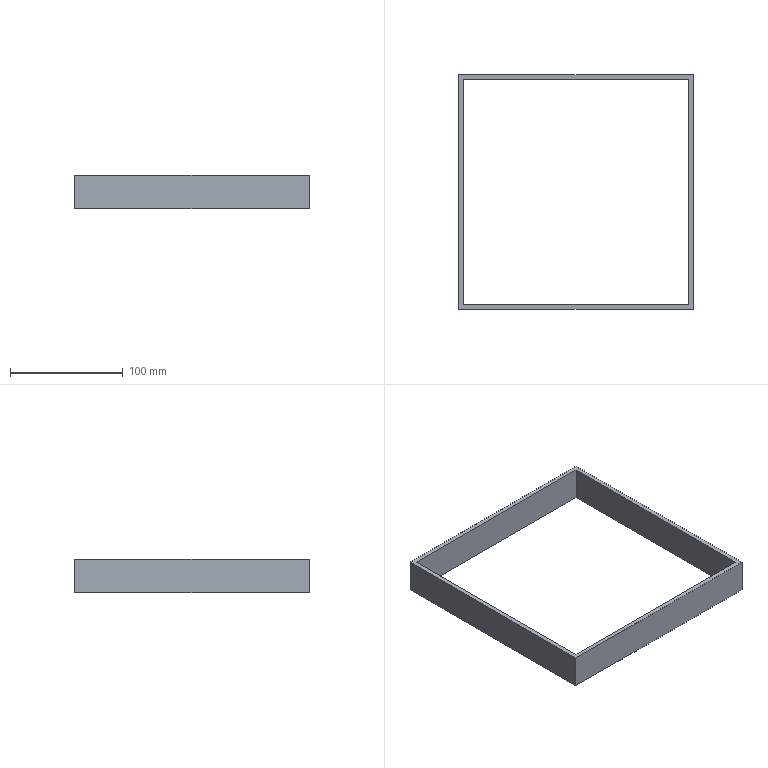Part | SolidWorks | features ExtruThin 1 | 1 solid | 10 faces | box 208 x 208 x 30 mm | volume 97920 mm3 | plane 10
STEP:
#1=CARTESIAN_POINT('',(-104.,104.,30.));
#2=VERTEX_POINT('',#1);
#3=CARTESIAN_POINT('',(-104.,-104.,30.));
#4=VERTEX_POINT('',#3);
#5=CARTESIAN_POINT('',(-104.,-100.,30.));
#6=DIRECTION('',(0.,-1.,0.));
#7=VECTOR('',#6,1000.);
#8=LINE('',#5,#7);
#9=EDGE_CURVE('',#2,#4,#8,.T.);
#10=ORIENTED_EDGE('',*,*,#9,.T.);
#11=CARTESIAN_POINT('',(104.,-104.,30.));
#12=VERTEX_POINT('',#11);
#13=CARTESIAN_POINT('',(100.,-104.,30.));
#14=DIRECTION('',(1.,0.,0.));
#15=VECTOR('',#14,1000.);
#16=LINE('',#13,#15);
#17=EDGE_CURVE('',#4,#12,#16,.T.);
#18=ORIENTED_EDGE('',*,*,#17,.T.);
#19=CARTESIAN_POINT('',(104.,104.,30.));
#20=VERTEX_POINT('',#19);
#21=CARTESIAN_POINT('',(104.,-100.,30.));
#22=DIRECTION('',(0.,1.,0.));
#23=VECTOR('',#22,1000.);
#24=LINE('',#21,#23);
#25=EDGE_CURVE('',#12,#20,#24,.T.);
#26=ORIENTED_EDGE('',*,*,#25,.T.);
#27=CARTESIAN_POINT('',(100.,104.,30.));
#28=DIRECTION('',(-1.,0.,0.));
#29=VECTOR('',#28,1000.);
#30=LINE('',#27,#29);
#31=EDGE_CURVE('',#20,#2,#30,.T.);
#32=ORIENTED_EDGE('',*,*,#31,.T.);
#33=EDGE_LOOP('',(#10,#18,#26,#32));
#34=FACE_OUTER_BOUND('',#33,.T.);
#35=CARTESIAN_POINT('',(-100.,-100.,30.));
#36=VERTEX_POINT('',#35);
#37=CARTESIAN_POINT('',(100.,-100.,30.));
#38=VERTEX_POINT('',#37);
#39=CARTESIAN_POINT('',(100.,-100.,30.));
#40=DIRECTION('',(1.,0.,0.));
#41=VECTOR('',#40,1000.);
#42=LINE('',#39,#41);
#43=EDGE_CURVE('',#36,#38,#42,.T.);
#44=ORIENTED_EDGE('',*,*,#43,.F.);
#45=CARTESIAN_POINT('',(-100.,100.,30.));
#46=VERTEX_POINT('',#45);
#47=CARTESIAN_POINT('',(-100.,-100.,30.));
#48=DIRECTION('',(0.,-1.,0.));
#49=VECTOR('',#48,1000.);
#50=LINE('',#47,#49);
#51=EDGE_CURVE('',#46,#36,#50,.T.);
#52=ORIENTED_EDGE('',*,*,#51,.F.);
#53=CARTESIAN_POINT('',(100.,100.,30.));
#54=VERTEX_POINT('',#53);
#55=CARTESIAN_POINT('',(100.,100.,30.));
#56=DIRECTION('',(-1.,0.,0.));
#57=VECTOR('',#56,1000.);
#58=LINE('',#55,#57);
#59=EDGE_CURVE('',#54,#46,#58,.T.);
#60=ORIENTED_EDGE('',*,*,#59,.F.);
#61=CARTESIAN_POINT('',(100.,-100.,30.));
#62=DIRECTION('',(0.,1.,0.));
#63=VECTOR('',#62,1000.);
#64=LINE('',#61,#63);
#65=EDGE_CURVE('',#38,#54,#64,.T.);
#66=ORIENTED_EDGE('',*,*,#65,.F.);
#67=EDGE_LOOP('',(#44,#52,#60,#66));
#68=FACE_BOUND('',#67,.T.);
#69=CARTESIAN_POINT('',(0.,0.,30.));
#70=DIRECTION('',(0.,0.,1.));
#71=DIRECTION('',(1.,0.,0.));
#72=AXIS2_PLACEMENT_3D('',#69,#70,#71);
#73=PLANE('',#72);
#74=ADVANCED_FACE('',(#34,#68),#73,.T.);
#75=CARTESIAN_POINT('',(-104.,104.,0.));
#76=VERTEX_POINT('',#75);
#77=CARTESIAN_POINT('',(-104.,-104.,0.));
#78=VERTEX_POINT('',#77);
#79=CARTESIAN_POINT('',(-104.,-100.,0.));
#80=DIRECTION('',(0.,-1.,0.));
#81=VECTOR('',#80,1000.);
#82=LINE('',#79,#81);
#83=EDGE_CURVE('',#76,#78,#82,.T.);
#84=ORIENTED_EDGE('',*,*,#83,.F.);
#85=CARTESIAN_POINT('',(104.,104.,0.));
#86=VERTEX_POINT('',#85);
#87=CARTESIAN_POINT('',(100.,104.,0.));
#88=DIRECTION('',(-1.,0.,0.));
#89=VECTOR('',#88,1000.);
#90=LINE('',#87,#89);
#91=EDGE_CURVE('',#86,#76,#90,.T.);
#92=ORIENTED_EDGE('',*,*,#91,.F.);
#93=CARTESIAN_POINT('',(104.,-104.,0.));
#94=VERTEX_POINT('',#93);
#95=CARTESIAN_POINT('',(104.,-100.,0.));
#96=DIRECTION('',(0.,1.,0.));
#97=VECTOR('',#96,1000.);
#98=LINE('',#95,#97);
#99=EDGE_CURVE('',#94,#86,#98,.T.);
#100=ORIENTED_EDGE('',*,*,#99,.F.);
#101=CARTESIAN_POINT('',(100.,-104.,0.));
#102=DIRECTION('',(1.,0.,0.));
#103=VECTOR('',#102,1000.);
#104=LINE('',#101,#103);
#105=EDGE_CURVE('',#78,#94,#104,.T.);
#106=ORIENTED_EDGE('',*,*,#105,.F.);
#107=EDGE_LOOP('',(#84,#92,#100,#106));
#108=FACE_OUTER_BOUND('',#107,.T.);
#109=CARTESIAN_POINT('',(-100.,100.,0.));
#110=VERTEX_POINT('',#109);
#111=CARTESIAN_POINT('',(-100.,-100.,0.));
#112=VERTEX_POINT('',#111);
#113=CARTESIAN_POINT('',(-100.,-100.,0.));
#114=DIRECTION('',(0.,-1.,0.));
#115=VECTOR('',#114,1000.);
#116=LINE('',#113,#115);
#117=EDGE_CURVE('',#110,#112,#116,.T.);
#118=ORIENTED_EDGE('',*,*,#117,.T.);
#119=CARTESIAN_POINT('',(100.,-100.,0.));
#120=VERTEX_POINT('',#119);
#121=CARTESIAN_POINT('',(100.,-100.,0.));
#122=DIRECTION('',(1.,0.,0.));
#123=VECTOR('',#122,1000.);
#124=LINE('',#121,#123);
#125=EDGE_CURVE('',#112,#120,#124,.T.);
#126=ORIENTED_EDGE('',*,*,#125,.T.);
#127=CARTESIAN_POINT('',(100.,100.,0.));
#128=VERTEX_POINT('',#127);
#129=CARTESIAN_POINT('',(100.,-100.,0.));
#130=DIRECTION('',(0.,1.,0.));
#131=VECTOR('',#130,1000.);
#132=LINE('',#129,#131);
#133=EDGE_CURVE('',#120,#128,#132,.T.);
#134=ORIENTED_EDGE('',*,*,#133,.T.);
#135=CARTESIAN_POINT('',(100.,100.,0.));
#136=DIRECTION('',(-1.,0.,0.));
#137=VECTOR('',#136,1000.);
#138=LINE('',#135,#137);
#139=EDGE_CURVE('',#128,#110,#138,.T.);
#140=ORIENTED_EDGE('',*,*,#139,.T.);
#141=EDGE_LOOP('',(#118,#126,#134,#140));
#142=FACE_BOUND('',#141,.T.);
#143=CARTESIAN_POINT('',(0.,0.,0.));
#144=DIRECTION('',(0.,0.,1.));
#145=DIRECTION('',(1.,0.,0.));
#146=AXIS2_PLACEMENT_3D('',#143,#144,#145);
#147=PLANE('',#146);
#148=ADVANCED_FACE('',(#108,#142),#147,.F.);
#149=ORIENTED_EDGE('',*,*,#83,.T.);
#150=CARTESIAN_POINT('',(-104.,-104.,30.));
#151=DIRECTION('',(0.,0.,-1.));
#152=VECTOR('',#151,1000.);
#153=LINE('',#150,#152);
#154=EDGE_CURVE('',#4,#78,#153,.T.);
#155=ORIENTED_EDGE('',*,*,#154,.F.);
#156=ORIENTED_EDGE('',*,*,#9,.F.);
#157=CARTESIAN_POINT('',(-104.,104.,30.));
#158=DIRECTION('',(0.,0.,-1.));
#159=VECTOR('',#158,1000.);
#160=LINE('',#157,#159);
#161=EDGE_CURVE('',#2,#76,#160,.T.);
#162=ORIENTED_EDGE('',*,*,#161,.T.);
#163=EDGE_LOOP('',(#149,#155,#156,#162));
#164=FACE_OUTER_BOUND('',#163,.T.);
#165=CARTESIAN_POINT('',(-104.,-100.,30.));
#166=DIRECTION('',(1.,0.,0.));
#167=DIRECTION('',(0.,0.,-1.));
#168=AXIS2_PLACEMENT_3D('',#165,#166,#167);
#169=PLANE('',#168);
#170=ADVANCED_FACE('',(#164),#169,.F.);
#171=ORIENTED_EDGE('',*,*,#105,.T.);
#172=CARTESIAN_POINT('',(104.,-104.,30.));
#173=DIRECTION('',(0.,0.,-1.));
#174=VECTOR('',#173,1000.);
#175=LINE('',#172,#174);
#176=EDGE_CURVE('',#12,#94,#175,.T.);
#177=ORIENTED_EDGE('',*,*,#176,.F.);
#178=ORIENTED_EDGE('',*,*,#17,.F.);
#179=ORIENTED_EDGE('',*,*,#154,.T.);
#180=EDGE_LOOP('',(#171,#177,#178,#179));
#181=FACE_OUTER_BOUND('',#180,.T.);
#182=CARTESIAN_POINT('',(100.,-104.,30.));
#183=DIRECTION('',(0.,1.,0.));
#184=DIRECTION('',(-1.,0.,0.));
#185=AXIS2_PLACEMENT_3D('',#182,#183,#184);
#186=PLANE('',#185);
#187=ADVANCED_FACE('',(#181),#186,.F.);
#188=ORIENTED_EDGE('',*,*,#99,.T.);
#189=CARTESIAN_POINT('',(104.,104.,30.));
#190=DIRECTION('',(0.,0.,-1.));
#191=VECTOR('',#190,1000.);
#192=LINE('',#189,#191);
#193=EDGE_CURVE('',#20,#86,#192,.T.);
#194=ORIENTED_EDGE('',*,*,#193,.F.);
#195=ORIENTED_EDGE('',*,*,#25,.F.);
#196=ORIENTED_EDGE('',*,*,#176,.T.);
#197=EDGE_LOOP('',(#188,#194,#195,#196));
#198=FACE_OUTER_BOUND('',#197,.T.);
#199=CARTESIAN_POINT('',(104.,-100.,30.));
#200=DIRECTION('',(-1.,0.,0.));
#201=DIRECTION('',(0.,0.,1.));
#202=AXIS2_PLACEMENT_3D('',#199,#200,#201);
#203=PLANE('',#202);
#204=ADVANCED_FACE('',(#198),#203,.F.);
#205=ORIENTED_EDGE('',*,*,#91,.T.);
#206=ORIENTED_EDGE('',*,*,#161,.F.);
#207=ORIENTED_EDGE('',*,*,#31,.F.);
#208=ORIENTED_EDGE('',*,*,#193,.T.);
#209=EDGE_LOOP('',(#205,#206,#207,#208));
#210=FACE_OUTER_BOUND('',#209,.T.);
#211=CARTESIAN_POINT('',(100.,104.,30.));
#212=DIRECTION('',(0.,-1.,0.));
#213=DIRECTION('',(1.,0.,0.));
#214=AXIS2_PLACEMENT_3D('',#211,#212,#213);
#215=PLANE('',#214);
#216=ADVANCED_FACE('',(#210),#215,.F.);
#217=ORIENTED_EDGE('',*,*,#117,.F.);
#218=CARTESIAN_POINT('',(-100.,100.,30.));
#219=DIRECTION('',(0.,0.,-1.));
#220=VECTOR('',#219,1000.);
#221=LINE('',#218,#220);
#222=EDGE_CURVE('',#46,#110,#221,.T.);
#223=ORIENTED_EDGE('',*,*,#222,.F.);
#224=ORIENTED_EDGE('',*,*,#51,.T.);
#225=CARTESIAN_POINT('',(-100.,-100.,30.));
#226=DIRECTION('',(0.,0.,-1.));
#227=VECTOR('',#226,1000.);
#228=LINE('',#225,#227);
#229=EDGE_CURVE('',#36,#112,#228,.T.);
#230=ORIENTED_EDGE('',*,*,#229,.T.);
#231=EDGE_LOOP('',(#217,#223,#224,#230));
#232=FACE_OUTER_BOUND('',#231,.T.);
#233=CARTESIAN_POINT('',(-100.,-100.,30.));
#234=DIRECTION('',(1.,0.,0.));
#235=DIRECTION('',(0.,0.,-1.));
#236=AXIS2_PLACEMENT_3D('',#233,#234,#235);
#237=PLANE('',#236);
#238=ADVANCED_FACE('',(#232),#237,.T.);
#239=ORIENTED_EDGE('',*,*,#125,.F.);
#240=ORIENTED_EDGE('',*,*,#229,.F.);
#241=ORIENTED_EDGE('',*,*,#43,.T.);
#242=CARTESIAN_POINT('',(100.,-100.,30.));
#243=DIRECTION('',(0.,0.,-1.));
#244=VECTOR('',#243,1000.);
#245=LINE('',#242,#244);
#246=EDGE_CURVE('',#38,#120,#245,.T.);
#247=ORIENTED_EDGE('',*,*,#246,.T.);
#248=EDGE_LOOP('',(#239,#240,#241,#247));
#249=FACE_OUTER_BOUND('',#248,.T.);
#250=CARTESIAN_POINT('',(100.,-100.,30.));
#251=DIRECTION('',(0.,1.,0.));
#252=DIRECTION('',(-1.,0.,0.));
#253=AXIS2_PLACEMENT_3D('',#250,#251,#252);
#254=PLANE('',#253);
#255=ADVANCED_FACE('',(#249),#254,.T.);
#256=ORIENTED_EDGE('',*,*,#133,.F.);
#257=ORIENTED_EDGE('',*,*,#246,.F.);
#258=ORIENTED_EDGE('',*,*,#65,.T.);
#259=CARTESIAN_POINT('',(100.,100.,30.));
#260=DIRECTION('',(0.,0.,-1.));
#261=VECTOR('',#260,1000.);
#262=LINE('',#259,#261);
#263=EDGE_CURVE('',#54,#128,#262,.T.);
#264=ORIENTED_EDGE('',*,*,#263,.T.);
#265=EDGE_LOOP('',(#256,#257,#258,#264));
#266=FACE_OUTER_BOUND('',#265,.T.);
#267=CARTESIAN_POINT('',(100.,-100.,30.));
#268=DIRECTION('',(-1.,0.,0.));
#269=DIRECTION('',(0.,0.,1.));
#270=AXIS2_PLACEMENT_3D('',#267,#268,#269);
#271=PLANE('',#270);
#272=ADVANCED_FACE('',(#266),#271,.T.);
#273=ORIENTED_EDGE('',*,*,#139,.F.);
#274=ORIENTED_EDGE('',*,*,#263,.F.);
#275=ORIENTED_EDGE('',*,*,#59,.T.);
#276=ORIENTED_EDGE('',*,*,#222,.T.);
#277=EDGE_LOOP('',(#273,#274,#275,#276));
#278=FACE_OUTER_BOUND('',#277,.T.);
#279=CARTESIAN_POINT('',(100.,100.,30.));
#280=DIRECTION('',(0.,-1.,0.));
#281=DIRECTION('',(1.,0.,0.));
#282=AXIS2_PLACEMENT_3D('',#279,#280,#281);
#283=PLANE('',#282);
#284=ADVANCED_FACE('',(#278),#283,.T.);
#285=CLOSED_SHELL('',(#74,#148,#170,#187,#204,#216,#238,#255,#272,#284));
#286=MANIFOLD_SOLID_BREP('',#285);
#287=CARTESIAN_POINT('',(0.,0.,0.));
#288=DIRECTION('',(0.,0.,1.));
#289=DIRECTION('',(1.,0.,0.));
#290=AXIS2_PLACEMENT_3D('',#287,#288,#289);
#291=(LENGTH_UNIT()NAMED_UNIT(*)SI_UNIT(.MILLI.,.METRE.));
#292=UNCERTAINTY_MEASURE_WITH_UNIT(LENGTH_MEASURE(0.00001),#291,'','');
#293=(NAMED_UNIT(*)PLANE_ANGLE_UNIT()SI_UNIT($,.RADIAN.));
#294=(NAMED_UNIT(*)SI_UNIT($,.STERADIAN.)SOLID_ANGLE_UNIT());
#295=(GEOMETRIC_REPRESENTATION_CONTEXT(3)GLOBAL_UNCERTAINTY_ASSIGNED_CONTEXT((#292))GLOBAL_UNIT_ASSIGNED_CONTEXT((#291,#293,#294))REPRESENTATION_CONTEXT('',''));
#296=ADVANCED_BREP_SHAPE_REPRESENTATION('',(#286,#290),#295);